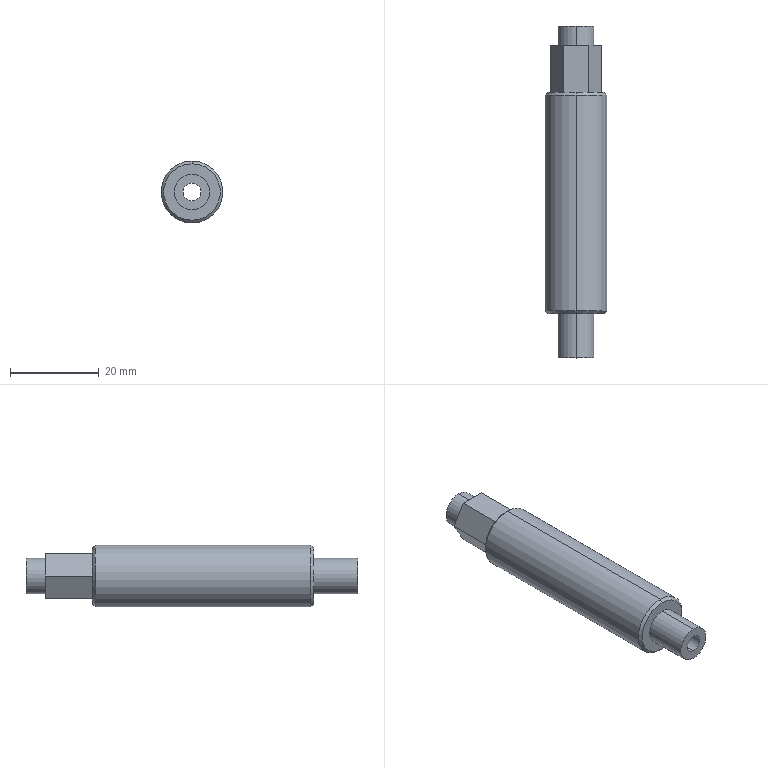Part | SolidWorks | features RefAxis 9, 3DProfileFeature 3, Revolution 2, ICE 1, RevCut 1 | 1 solid | 29 faces | box 14 x 75 x 14 mm | volume 8378 mm3 | plane 11 | cylinder 10 | cone 8 | commonest cylinder face diameters 8 x4 4 x2 4.134 x2 14 x2
STEP:
#1=CARTESIAN_POINT('',(0.,50.,-2.));
#2=VERTEX_POINT('',#1);
#3=CARTESIAN_POINT('',(0.,50.,2.));
#4=VERTEX_POINT('',#3);
#5=CARTESIAN_POINT('',(0.,50.,0.));
#6=DIRECTION('',(0.,1.,0.));
#7=DIRECTION('',(0.,0.,1.));
#8=AXIS2_PLACEMENT_3D('',#5,#6,#7);
#9=CIRCLE('',#8,2.);
#10=EDGE_CURVE('',#2,#4,#9,.T.);
#11=ORIENTED_EDGE('',*,*,#10,.F.);
#12=CARTESIAN_POINT('',(0.,119.961,-2.));
#13=VERTEX_POINT('',#12);
#14=CARTESIAN_POINT('',(0.,50.,-2.));
#15=DIRECTION('',(0.,1.,0.));
#16=VECTOR('',#15,1000.);
#17=LINE('',#14,#16);
#18=EDGE_CURVE('',#2,#13,#17,.T.);
#19=ORIENTED_EDGE('',*,*,#18,.T.);
#20=CARTESIAN_POINT('',(0.,119.961,2.));
#21=VERTEX_POINT('',#20);
#22=CARTESIAN_POINT('',(0.,119.961,0.));
#23=DIRECTION('',(0.,1.,0.));
#24=DIRECTION('',(0.,0.,1.));
#25=AXIS2_PLACEMENT_3D('',#22,#23,#24);
#26=CIRCLE('',#25,2.);
#27=EDGE_CURVE('',#13,#21,#26,.T.);
#28=ORIENTED_EDGE('',*,*,#27,.T.);
#29=CARTESIAN_POINT('',(0.,50.,2.));
#30=DIRECTION('',(0.,1.,0.));
#31=VECTOR('',#30,1000.);
#32=LINE('',#29,#31);
#33=EDGE_CURVE('',#4,#21,#32,.T.);
#34=ORIENTED_EDGE('',*,*,#33,.F.);
#35=EDGE_LOOP('',(#11,#19,#28,#34));
#36=FACE_OUTER_BOUND('',#35,.T.);
#37=CARTESIAN_POINT('',(0.,50.,0.));
#38=DIRECTION('',(0.,1.,0.));
#39=DIRECTION('',(0.,0.,1.));
#40=AXIS2_PLACEMENT_3D('',#37,#38,#39);
#41=CYLINDRICAL_SURFACE('',#40,2.);
#42=ADVANCED_FACE('',(#36),#41,.F.);
#43=ORIENTED_EDGE('',*,*,#27,.F.);
#44=CARTESIAN_POINT('',(0.,120.,-2.067));
#45=VERTEX_POINT('',#44);
#46=CARTESIAN_POINT('',(0.,119.961,-2.));
#47=DIRECTION('',(0.,0.5,-0.866));
#48=VECTOR('',#47,1000.);
#49=LINE('',#46,#48);
#50=EDGE_CURVE('',#13,#45,#49,.T.);
#51=ORIENTED_EDGE('',*,*,#50,.T.);
#52=CARTESIAN_POINT('',(0.,120.,2.067));
#53=VERTEX_POINT('',#52);
#54=CARTESIAN_POINT('',(0.,120.,0.));
#55=DIRECTION('',(0.,1.,0.));
#56=DIRECTION('',(0.,0.,1.));
#57=AXIS2_PLACEMENT_3D('',#54,#55,#56);
#58=CIRCLE('',#57,2.067);
#59=EDGE_CURVE('',#45,#53,#58,.T.);
#60=ORIENTED_EDGE('',*,*,#59,.T.);
#61=CARTESIAN_POINT('',(0.,119.961,2.));
#62=DIRECTION('',(0.,0.5,0.866));
#63=VECTOR('',#62,1000.);
#64=LINE('',#61,#63);
#65=EDGE_CURVE('',#21,#53,#64,.T.);
#66=ORIENTED_EDGE('',*,*,#65,.F.);
#67=EDGE_LOOP('',(#43,#51,#60,#66));
#68=FACE_OUTER_BOUND('',#67,.T.);
#69=CARTESIAN_POINT('',(0.,119.961,0.));
#70=DIRECTION('',(0.,1.,0.));
#71=DIRECTION('',(0.,0.,1.));
#72=AXIS2_PLACEMENT_3D('',#69,#70,#71);
#73=CONICAL_SURFACE('',#72,2.,1.047);
#74=ADVANCED_FACE('',(#68),#73,.F.);
#75=ORIENTED_EDGE('',*,*,#59,.F.);
#76=CARTESIAN_POINT('',(0.,124.567,-2.067));
#77=VERTEX_POINT('',#76);
#78=CARTESIAN_POINT('',(0.,50.,-2.067));
#79=DIRECTION('',(0.,1.,0.));
#80=VECTOR('',#79,1000.);
#81=LINE('',#78,#80);
#82=EDGE_CURVE('',#45,#77,#81,.T.);
#83=ORIENTED_EDGE('',*,*,#82,.T.);
#84=CARTESIAN_POINT('',(0.,124.567,2.067));
#85=VERTEX_POINT('',#84);
#86=CARTESIAN_POINT('',(0.,124.567,0.));
#87=DIRECTION('',(0.,1.,0.));
#88=DIRECTION('',(0.,0.,1.));
#89=AXIS2_PLACEMENT_3D('',#86,#87,#88);
#90=CIRCLE('',#89,2.067);
#91=EDGE_CURVE('',#77,#85,#90,.T.);
#92=ORIENTED_EDGE('',*,*,#91,.T.);
#93=CARTESIAN_POINT('',(0.,50.,2.067));
#94=DIRECTION('',(0.,1.,0.));
#95=VECTOR('',#94,1000.);
#96=LINE('',#93,#95);
#97=EDGE_CURVE('',#53,#85,#96,.T.);
#98=ORIENTED_EDGE('',*,*,#97,.F.);
#99=EDGE_LOOP('',(#75,#83,#92,#98));
#100=FACE_OUTER_BOUND('',#99,.T.);
#101=CARTESIAN_POINT('',(0.,50.,0.));
#102=DIRECTION('',(0.,1.,0.));
#103=DIRECTION('',(0.,0.,1.));
#104=AXIS2_PLACEMENT_3D('',#101,#102,#103);
#105=CYLINDRICAL_SURFACE('',#104,2.067);
#106=ADVANCED_FACE('',(#100),#105,.F.);
#107=ORIENTED_EDGE('',*,*,#91,.F.);
#108=CARTESIAN_POINT('',(0.,125.,-2.5));
#109=VERTEX_POINT('',#108);
#110=CARTESIAN_POINT('',(0.,124.567,-2.067));
#111=DIRECTION('',(0.,0.7071,-0.7071));
#112=VECTOR('',#111,1000.);
#113=LINE('',#110,#112);
#114=EDGE_CURVE('',#77,#109,#113,.T.);
#115=ORIENTED_EDGE('',*,*,#114,.T.);
#116=CARTESIAN_POINT('',(0.,125.,2.5));
#117=VERTEX_POINT('',#116);
#118=CARTESIAN_POINT('',(0.,125.,0.));
#119=DIRECTION('',(0.,1.,0.));
#120=DIRECTION('',(0.,0.,1.));
#121=AXIS2_PLACEMENT_3D('',#118,#119,#120);
#122=CIRCLE('',#121,2.5);
#123=EDGE_CURVE('',#109,#117,#122,.T.);
#124=ORIENTED_EDGE('',*,*,#123,.T.);
#125=CARTESIAN_POINT('',(0.,124.567,2.067));
#126=DIRECTION('',(0.,0.7071,0.7071));
#127=VECTOR('',#126,1000.);
#128=LINE('',#125,#127);
#129=EDGE_CURVE('',#85,#117,#128,.T.);
#130=ORIENTED_EDGE('',*,*,#129,.F.);
#131=EDGE_LOOP('',(#107,#115,#124,#130));
#132=FACE_OUTER_BOUND('',#131,.T.);
#133=CARTESIAN_POINT('',(0.,124.567,0.));
#134=DIRECTION('',(0.,1.,0.));
#135=DIRECTION('',(0.,0.,1.));
#136=AXIS2_PLACEMENT_3D('',#133,#134,#135);
#137=CONICAL_SURFACE('',#136,2.067,0.7854);
#138=ADVANCED_FACE('',(#132),#137,.F.);
#139=CARTESIAN_POINT('',(0.,120.7,4.));
#140=VERTEX_POINT('',#139);
#141=CARTESIAN_POINT('',(0.,120.7,-4.));
#142=VERTEX_POINT('',#141);
#143=CARTESIAN_POINT('',(0.,120.7,0.));
#144=DIRECTION('',(0.,1.,0.));
#145=DIRECTION('',(0.,0.,1.));
#146=AXIS2_PLACEMENT_3D('',#143,#144,#145);
#147=CIRCLE('',#146,4.);
#148=EDGE_CURVE('',#140,#142,#147,.T.);
#149=ORIENTED_EDGE('',*,*,#148,.T.);
#150=CARTESIAN_POINT('',(0.,125.,-4.));
#151=VERTEX_POINT('',#150);
#152=CARTESIAN_POINT('',(0.,120.7,-4.));
#153=DIRECTION('',(0.,1.,0.));
#154=VECTOR('',#153,1000.);
#155=LINE('',#152,#154);
#156=EDGE_CURVE('',#142,#151,#155,.T.);
#157=ORIENTED_EDGE('',*,*,#156,.T.);
#158=CARTESIAN_POINT('',(0.,125.,4.));
#159=VERTEX_POINT('',#158);
#160=CARTESIAN_POINT('',(0.,125.,0.));
#161=DIRECTION('',(0.,1.,0.));
#162=DIRECTION('',(0.,0.,1.));
#163=AXIS2_PLACEMENT_3D('',#160,#161,#162);
#164=CIRCLE('',#163,4.);
#165=EDGE_CURVE('',#159,#151,#164,.T.);
#166=ORIENTED_EDGE('',*,*,#165,.F.);
#167=CARTESIAN_POINT('',(0.,120.7,4.));
#168=DIRECTION('',(0.,1.,0.));
#169=VECTOR('',#168,1000.);
#170=LINE('',#167,#169);
#171=EDGE_CURVE('',#140,#159,#170,.T.);
#172=ORIENTED_EDGE('',*,*,#171,.F.);
#173=EDGE_LOOP('',(#149,#157,#166,#172));
#174=FACE_OUTER_BOUND('',#173,.T.);
#175=CARTESIAN_POINT('',(0.,120.7,0.));
#176=DIRECTION('',(0.,1.,0.));
#177=DIRECTION('',(0.,0.,1.));
#178=AXIS2_PLACEMENT_3D('',#175,#176,#177);
#179=CYLINDRICAL_SURFACE('',#178,4.);
#180=ADVANCED_FACE('',(#174),#179,.T.);
#181=CARTESIAN_POINT('',(0.,50.,4.));
#182=VERTEX_POINT('',#181);
#183=CARTESIAN_POINT('',(0.,50.,-4.));
#184=VERTEX_POINT('',#183);
#185=CARTESIAN_POINT('',(0.,50.,0.));
#186=DIRECTION('',(0.,1.,0.));
#187=DIRECTION('',(0.,0.,1.));
#188=AXIS2_PLACEMENT_3D('',#185,#186,#187);
#189=CIRCLE('',#188,4.);
#190=EDGE_CURVE('',#182,#184,#189,.T.);
#191=ORIENTED_EDGE('',*,*,#190,.T.);
#192=CARTESIAN_POINT('',(0.,60.,-4.));
#193=VERTEX_POINT('',#192);
#194=CARTESIAN_POINT('',(0.,50.,-4.));
#195=DIRECTION('',(0.,1.,0.));
#196=VECTOR('',#195,1000.);
#197=LINE('',#194,#196);
#198=EDGE_CURVE('',#184,#193,#197,.T.);
#199=ORIENTED_EDGE('',*,*,#198,.T.);
#200=CARTESIAN_POINT('',(0.,60.,4.));
#201=VERTEX_POINT('',#200);
#202=CARTESIAN_POINT('',(0.,60.,0.));
#203=DIRECTION('',(0.,1.,0.));
#204=DIRECTION('',(0.,0.,1.));
#205=AXIS2_PLACEMENT_3D('',#202,#203,#204);
#206=CIRCLE('',#205,4.);
#207=EDGE_CURVE('',#201,#193,#206,.T.);
#208=ORIENTED_EDGE('',*,*,#207,.F.);
#209=CARTESIAN_POINT('',(0.,50.,4.));
#210=DIRECTION('',(0.,1.,0.));
#211=VECTOR('',#210,1000.);
#212=LINE('',#209,#211);
#213=EDGE_CURVE('',#182,#201,#212,.T.);
#214=ORIENTED_EDGE('',*,*,#213,.F.);
#215=EDGE_LOOP('',(#191,#199,#208,#214));
#216=FACE_OUTER_BOUND('',#215,.T.);
#217=CARTESIAN_POINT('',(0.,50.,0.));
#218=DIRECTION('',(0.,1.,0.));
#219=DIRECTION('',(0.,0.,1.));
#220=AXIS2_PLACEMENT_3D('',#217,#218,#219);
#221=CYLINDRICAL_SURFACE('',#220,4.);
#222=ADVANCED_FACE('',(#216),#221,.T.);
#223=CARTESIAN_POINT('',(0.,60.,6.386));
#224=VERTEX_POINT('',#223);
#225=CARTESIAN_POINT('',(0.,60.,-6.386));
#226=VERTEX_POINT('',#225);
#227=CARTESIAN_POINT('',(0.,60.,0.));
#228=DIRECTION('',(0.,1.,0.));
#229=DIRECTION('',(0.,0.,1.));
#230=AXIS2_PLACEMENT_3D('',#227,#228,#229);
#231=CIRCLE('',#230,6.386);
#232=EDGE_CURVE('',#224,#226,#231,.T.);
#233=ORIENTED_EDGE('',*,*,#232,.T.);
#234=CARTESIAN_POINT('',(0.,60.614,-7.));
#235=VERTEX_POINT('',#234);
#236=CARTESIAN_POINT('',(0.,60.,-6.386));
#237=DIRECTION('',(0.,0.7071,-0.7071));
#238=VECTOR('',#237,1000.);
#239=LINE('',#236,#238);
#240=EDGE_CURVE('',#226,#235,#239,.T.);
#241=ORIENTED_EDGE('',*,*,#240,.T.);
#242=CARTESIAN_POINT('',(0.,60.614,7.));
#243=VERTEX_POINT('',#242);
#244=CARTESIAN_POINT('',(0.,60.614,0.));
#245=DIRECTION('',(0.,1.,0.));
#246=DIRECTION('',(0.,0.,1.));
#247=AXIS2_PLACEMENT_3D('',#244,#245,#246);
#248=CIRCLE('',#247,7.);
#249=EDGE_CURVE('',#243,#235,#248,.T.);
#250=ORIENTED_EDGE('',*,*,#249,.F.);
#251=CARTESIAN_POINT('',(0.,60.,6.386));
#252=DIRECTION('',(0.,0.7071,0.7071));
#253=VECTOR('',#252,1000.);
#254=LINE('',#251,#253);
#255=EDGE_CURVE('',#224,#243,#254,.T.);
#256=ORIENTED_EDGE('',*,*,#255,.F.);
#257=EDGE_LOOP('',(#233,#241,#250,#256));
#258=FACE_OUTER_BOUND('',#257,.T.);
#259=CARTESIAN_POINT('',(0.,60.,0.));
#260=DIRECTION('',(0.,1.,0.));
#261=DIRECTION('',(0.,0.,1.));
#262=AXIS2_PLACEMENT_3D('',#259,#260,#261);
#263=CONICAL_SURFACE('',#262,6.386,0.7854);
#264=ADVANCED_FACE('',(#258),#263,.T.);
#265=ORIENTED_EDGE('',*,*,#249,.T.);
#266=CARTESIAN_POINT('',(0.,109.386,-7.));
#267=VERTEX_POINT('',#266);
#268=CARTESIAN_POINT('',(0.,50.,-7.));
#269=DIRECTION('',(0.,1.,0.));
#270=VECTOR('',#269,1000.);
#271=LINE('',#268,#270);
#272=EDGE_CURVE('',#235,#267,#271,.T.);
#273=ORIENTED_EDGE('',*,*,#272,.T.);
#274=CARTESIAN_POINT('',(0.,109.386,7.));
#275=VERTEX_POINT('',#274);
#276=CARTESIAN_POINT('',(0.,109.386,0.));
#277=DIRECTION('',(0.,1.,0.));
#278=DIRECTION('',(0.,0.,1.));
#279=AXIS2_PLACEMENT_3D('',#276,#277,#278);
#280=CIRCLE('',#279,7.);
#281=EDGE_CURVE('',#275,#267,#280,.T.);
#282=ORIENTED_EDGE('',*,*,#281,.F.);
#283=CARTESIAN_POINT('',(0.,50.,7.));
#284=DIRECTION('',(0.,1.,0.));
#285=VECTOR('',#284,1000.);
#286=LINE('',#283,#285);
#287=EDGE_CURVE('',#243,#275,#286,.T.);
#288=ORIENTED_EDGE('',*,*,#287,.F.);
#289=EDGE_LOOP('',(#265,#273,#282,#288));
#290=FACE_OUTER_BOUND('',#289,.T.);
#291=CARTESIAN_POINT('',(0.,50.,0.));
#292=DIRECTION('',(0.,1.,0.));
#293=DIRECTION('',(0.,0.,1.));
#294=AXIS2_PLACEMENT_3D('',#291,#292,#293);
#295=CYLINDRICAL_SURFACE('',#294,7.);
#296=ADVANCED_FACE('',(#290),#295,.T.);
#297=CARTESIAN_POINT('',(0.,110.,6.386));
#298=VERTEX_POINT('',#297);
#299=CARTESIAN_POINT('',(0.,110.,-6.386));
#300=VERTEX_POINT('',#299);
#301=CARTESIAN_POINT('',(0.,110.,0.));
#302=DIRECTION('',(0.,1.,0.));
#303=DIRECTION('',(0.,0.,1.));
#304=AXIS2_PLACEMENT_3D('',#301,#302,#303);
#305=CIRCLE('',#304,6.386);
#306=EDGE_CURVE('',#298,#300,#305,.T.);
#307=ORIENTED_EDGE('',*,*,#306,.F.);
#308=CARTESIAN_POINT('',(0.,109.386,7.));
#309=DIRECTION('',(0.,-0.7071,0.7071));
#310=VECTOR('',#309,1000.);
#311=LINE('',#308,#310);
#312=EDGE_CURVE('',#298,#275,#311,.T.);
#313=ORIENTED_EDGE('',*,*,#312,.T.);
#314=ORIENTED_EDGE('',*,*,#281,.T.);
#315=CARTESIAN_POINT('',(0.,109.386,-7.));
#316=DIRECTION('',(0.,-0.7071,-0.7071));
#317=VECTOR('',#316,1000.);
#318=LINE('',#315,#317);
#319=EDGE_CURVE('',#300,#267,#318,.T.);
#320=ORIENTED_EDGE('',*,*,#319,.F.);
#321=EDGE_LOOP('',(#307,#313,#314,#320));
#322=FACE_OUTER_BOUND('',#321,.T.);
#323=CARTESIAN_POINT('',(0.,109.386,0.));
#324=DIRECTION('',(0.,-1.,0.));
#325=DIRECTION('',(0.,0.,-1.));
#326=AXIS2_PLACEMENT_3D('',#323,#324,#325);
#327=CONICAL_SURFACE('',#326,7.,0.7854);
#328=ADVANCED_FACE('',(#322),#327,.T.);
#329=ORIENTED_EDGE('',*,*,#190,.F.);
#330=CARTESIAN_POINT('',(0.,50.,0.));
#331=DIRECTION('',(0.,1.,0.));
#332=DIRECTION('',(0.,0.,1.));
#333=AXIS2_PLACEMENT_3D('',#330,#331,#332);
#334=CIRCLE('',#333,4.);
#335=EDGE_CURVE('',#184,#182,#334,.T.);
#336=ORIENTED_EDGE('',*,*,#335,.F.);
#337=EDGE_LOOP('',(#329,#336));
#338=FACE_OUTER_BOUND('',#337,.T.);
#339=CARTESIAN_POINT('',(0.,50.,0.));
#340=DIRECTION('',(0.,1.,0.));
#341=DIRECTION('',(0.,0.,1.));
#342=AXIS2_PLACEMENT_3D('',#339,#340,#341);
#343=CIRCLE('',#342,2.);
#344=EDGE_CURVE('',#4,#2,#343,.T.);
#345=ORIENTED_EDGE('',*,*,#344,.T.);
#346=ORIENTED_EDGE('',*,*,#10,.T.);
#347=EDGE_LOOP('',(#345,#346));
#348=FACE_BOUND('',#347,.T.);
#349=CARTESIAN_POINT('',(4.,50.,0.));
#350=DIRECTION('',(0.,1.,0.));
#351=DIRECTION('',(0.,0.,1.));
#352=AXIS2_PLACEMENT_3D('',#349,#350,#351);
#353=PLANE('',#352);
#354=ADVANCED_FACE('',(#338,#348),#353,.F.);
#355=ORIENTED_EDGE('',*,*,#165,.T.);
#356=CARTESIAN_POINT('',(0.,125.,0.));
#357=DIRECTION('',(0.,1.,0.));
#358=DIRECTION('',(0.,0.,1.));
#359=AXIS2_PLACEMENT_3D('',#356,#357,#358);
#360=CIRCLE('',#359,4.);
#361=EDGE_CURVE('',#151,#159,#360,.T.);
#362=ORIENTED_EDGE('',*,*,#361,.T.);
#363=EDGE_LOOP('',(#355,#362));
#364=FACE_OUTER_BOUND('',#363,.T.);
#365=CARTESIAN_POINT('',(0.,125.,0.));
#366=DIRECTION('',(0.,1.,0.));
#367=DIRECTION('',(0.,0.,1.));
#368=AXIS2_PLACEMENT_3D('',#365,#366,#367);
#369=CIRCLE('',#368,2.5);
#370=EDGE_CURVE('',#117,#109,#369,.T.);
#371=ORIENTED_EDGE('',*,*,#370,.F.);
#372=ORIENTED_EDGE('',*,*,#123,.F.);
#373=EDGE_LOOP('',(#371,#372));
#374=FACE_BOUND('',#373,.T.);
#375=CARTESIAN_POINT('',(0.,125.,0.));
#376=DIRECTION('',(0.,-1.,0.));
#377=DIRECTION('',(0.,0.,-1.));
#378=AXIS2_PLACEMENT_3D('',#375,#376,#377);
#379=PLANE('',#378);
#380=ADVANCED_FACE('',(#364,#374),#379,.F.);
#381=CARTESIAN_POINT('',(-2.887,120.7,-5.));
#382=VERTEX_POINT('',#381);
#383=CARTESIAN_POINT('',(-5.774,120.7,0.));
#384=VERTEX_POINT('',#383);
#385=CARTESIAN_POINT('',(-2.887,120.7,-5.));
#386=DIRECTION('',(-0.5,0.,0.866));
#387=VECTOR('',#386,1000.);
#388=LINE('',#385,#387);
#389=EDGE_CURVE('',#382,#384,#388,.T.);
#390=ORIENTED_EDGE('',*,*,#389,.T.);
#391=CARTESIAN_POINT('',(-2.887,120.7,5.));
#392=VERTEX_POINT('',#391);
#393=CARTESIAN_POINT('',(-5.774,120.7,0.));
#394=DIRECTION('',(0.5,0.,0.866));
#395=VECTOR('',#394,1000.);
#396=LINE('',#393,#395);
#397=EDGE_CURVE('',#384,#392,#396,.T.);
#398=ORIENTED_EDGE('',*,*,#397,.T.);
#399=CARTESIAN_POINT('',(2.887,120.7,5.));
#400=VERTEX_POINT('',#399);
#401=CARTESIAN_POINT('',(-2.887,120.7,5.));
#402=DIRECTION('',(1.,0.,0.));
#403=VECTOR('',#402,1000.);
#404=LINE('',#401,#403);
#405=EDGE_CURVE('',#392,#400,#404,.T.);
#406=ORIENTED_EDGE('',*,*,#405,.T.);
#407=CARTESIAN_POINT('',(5.774,120.7,0.));
#408=VERTEX_POINT('',#407);
#409=CARTESIAN_POINT('',(2.887,120.7,5.));
#410=DIRECTION('',(0.5,0.,-0.866));
#411=VECTOR('',#410,1000.);
#412=LINE('',#409,#411);
#413=EDGE_CURVE('',#400,#408,#412,.T.);
#414=ORIENTED_EDGE('',*,*,#413,.T.);
#415=CARTESIAN_POINT('',(2.887,120.7,-5.));
#416=VERTEX_POINT('',#415);
#417=CARTESIAN_POINT('',(5.774,120.7,0.));
#418=DIRECTION('',(-0.5,0.,-0.866));
#419=VECTOR('',#418,1000.);
#420=LINE('',#417,#419);
#421=EDGE_CURVE('',#408,#416,#420,.T.);
#422=ORIENTED_EDGE('',*,*,#421,.T.);
#423=CARTESIAN_POINT('',(2.887,120.7,-5.));
#424=DIRECTION('',(-1.,0.,0.));
#425=VECTOR('',#424,1000.);
#426=LINE('',#423,#425);
#427=EDGE_CURVE('',#416,#382,#426,.T.);
#428=ORIENTED_EDGE('',*,*,#427,.T.);
#429=EDGE_LOOP('',(#390,#398,#406,#414,#422,#428));
#430=FACE_OUTER_BOUND('',#429,.T.);
#431=ORIENTED_EDGE('',*,*,#148,.F.);
#432=CARTESIAN_POINT('',(0.,120.7,0.));
#433=DIRECTION('',(0.,1.,0.));
#434=DIRECTION('',(0.,0.,1.));
#435=AXIS2_PLACEMENT_3D('',#432,#433,#434);
#436=CIRCLE('',#435,4.);
#437=EDGE_CURVE('',#142,#140,#436,.T.);
#438=ORIENTED_EDGE('',*,*,#437,.F.);
#439=EDGE_LOOP('',(#431,#438));
#440=FACE_BOUND('',#439,.T.);
#441=CARTESIAN_POINT('',(0.,120.7,0.));
#442=DIRECTION('',(0.,1.,0.));
#443=DIRECTION('',(0.,0.,1.));
#444=AXIS2_PLACEMENT_3D('',#441,#442,#443);
#445=PLANE('',#444);
#446=ADVANCED_FACE('',(#430,#440),#445,.T.);
#447=CARTESIAN_POINT('',(0.,110.,0.));
#448=DIRECTION('',(0.,1.,0.));
#449=DIRECTION('',(0.,0.,1.));
#450=AXIS2_PLACEMENT_3D('',#447,#448,#449);
#451=CIRCLE('',#450,6.386);
#452=EDGE_CURVE('',#300,#298,#451,.T.);
#453=ORIENTED_EDGE('',*,*,#452,.T.);
#454=ORIENTED_EDGE('',*,*,#306,.T.);
#455=EDGE_LOOP('',(#453,#454));
#456=FACE_OUTER_BOUND('',#455,.T.);
#457=CARTESIAN_POINT('',(-2.887,110.,-5.));
#458=VERTEX_POINT('',#457);
#459=CARTESIAN_POINT('',(-5.774,110.,0.));
#460=VERTEX_POINT('',#459);
#461=CARTESIAN_POINT('',(-2.887,110.,-5.));
#462=DIRECTION('',(-0.5,0.,0.866));
#463=VECTOR('',#462,1000.);
#464=LINE('',#461,#463);
#465=EDGE_CURVE('',#458,#460,#464,.T.);
#466=ORIENTED_EDGE('',*,*,#465,.F.);
#467=CARTESIAN_POINT('',(2.887,110.,-5.));
#468=VERTEX_POINT('',#467);
#469=CARTESIAN_POINT('',(2.887,110.,-5.));
#470=DIRECTION('',(-1.,0.,0.));
#471=VECTOR('',#470,1000.);
#472=LINE('',#469,#471);
#473=EDGE_CURVE('',#468,#458,#472,.T.);
#474=ORIENTED_EDGE('',*,*,#473,.F.);
#475=CARTESIAN_POINT('',(5.774,110.,0.));
#476=VERTEX_POINT('',#475);
#477=CARTESIAN_POINT('',(5.774,110.,0.));
#478=DIRECTION('',(-0.5,0.,-0.866));
#479=VECTOR('',#478,1000.);
#480=LINE('',#477,#479);
#481=EDGE_CURVE('',#476,#468,#480,.T.);
#482=ORIENTED_EDGE('',*,*,#481,.F.);
#483=CARTESIAN_POINT('',(2.887,110.,5.));
#484=VERTEX_POINT('',#483);
#485=CARTESIAN_POINT('',(2.887,110.,5.));
#486=DIRECTION('',(0.5,0.,-0.866));
#487=VECTOR('',#486,1000.);
#488=LINE('',#485,#487);
#489=EDGE_CURVE('',#484,#476,#488,.T.);
#490=ORIENTED_EDGE('',*,*,#489,.F.);
#491=CARTESIAN_POINT('',(-2.887,110.,5.));
#492=VERTEX_POINT('',#491);
#493=CARTESIAN_POINT('',(-2.887,110.,5.));
#494=DIRECTION('',(1.,0.,0.));
#495=VECTOR('',#494,1000.);
#496=LINE('',#493,#495);
#497=EDGE_CURVE('',#492,#484,#496,.T.);
#498=ORIENTED_EDGE('',*,*,#497,.F.);
#499=CARTESIAN_POINT('',(-5.774,110.,0.));
#500=DIRECTION('',(0.5,0.,0.866));
#501=VECTOR('',#500,1000.);
#502=LINE('',#499,#501);
#503=EDGE_CURVE('',#460,#492,#502,.T.);
#504=ORIENTED_EDGE('',*,*,#503,.F.);
#505=EDGE_LOOP('',(#466,#474,#482,#490,#498,#504));
#506=FACE_BOUND('',#505,.T.);
#507=CARTESIAN_POINT('',(0.,110.,0.));
#508=DIRECTION('',(0.,-1.,0.));
#509=DIRECTION('',(0.,0.,-1.));
#510=AXIS2_PLACEMENT_3D('',#507,#508,#509);
#511=PLANE('',#510);
#512=ADVANCED_FACE('',(#456,#506),#511,.F.);
#513=ORIENTED_EDGE('',*,*,#312,.F.);
#514=ORIENTED_EDGE('',*,*,#452,.F.);
#515=ORIENTED_EDGE('',*,*,#319,.T.);
#516=CARTESIAN_POINT('',(0.,109.386,0.));
#517=DIRECTION('',(0.,1.,0.));
#518=DIRECTION('',(0.,0.,1.));
#519=AXIS2_PLACEMENT_3D('',#516,#517,#518);
#520=CIRCLE('',#519,7.);
#521=EDGE_CURVE('',#267,#275,#520,.T.);
#522=ORIENTED_EDGE('',*,*,#521,.T.);
#523=EDGE_LOOP('',(#513,#514,#515,#522));
#524=FACE_OUTER_BOUND('',#523,.T.);
#525=CARTESIAN_POINT('',(0.,109.386,0.));
#526=DIRECTION('',(0.,-1.,0.));
#527=DIRECTION('',(0.,0.,-1.));
#528=AXIS2_PLACEMENT_3D('',#525,#526,#527);
#529=CONICAL_SURFACE('',#528,7.,0.7854);
#530=ADVANCED_FACE('',(#524),#529,.T.);
#531=ORIENTED_EDGE('',*,*,#272,.F.);
#532=CARTESIAN_POINT('',(0.,60.614,0.));
#533=DIRECTION('',(0.,1.,0.));
#534=DIRECTION('',(0.,0.,1.));
#535=AXIS2_PLACEMENT_3D('',#532,#533,#534);
#536=CIRCLE('',#535,7.);
#537=EDGE_CURVE('',#235,#243,#536,.T.);
#538=ORIENTED_EDGE('',*,*,#537,.T.);
#539=ORIENTED_EDGE('',*,*,#287,.T.);
#540=ORIENTED_EDGE('',*,*,#521,.F.);
#541=EDGE_LOOP('',(#531,#538,#539,#540));
#542=FACE_OUTER_BOUND('',#541,.T.);
#543=CARTESIAN_POINT('',(0.,50.,0.));
#544=DIRECTION('',(0.,1.,0.));
#545=DIRECTION('',(0.,0.,1.));
#546=AXIS2_PLACEMENT_3D('',#543,#544,#545);
#547=CYLINDRICAL_SURFACE('',#546,7.);
#548=ADVANCED_FACE('',(#542),#547,.T.);
#549=ORIENTED_EDGE('',*,*,#240,.F.);
#550=CARTESIAN_POINT('',(0.,60.,0.));
#551=DIRECTION('',(0.,1.,0.));
#552=DIRECTION('',(0.,0.,1.));
#553=AXIS2_PLACEMENT_3D('',#550,#551,#552);
#554=CIRCLE('',#553,6.386);
#555=EDGE_CURVE('',#226,#224,#554,.T.);
#556=ORIENTED_EDGE('',*,*,#555,.T.);
#557=ORIENTED_EDGE('',*,*,#255,.T.);
#558=ORIENTED_EDGE('',*,*,#537,.F.);
#559=EDGE_LOOP('',(#549,#556,#557,#558));
#560=FACE_OUTER_BOUND('',#559,.T.);
#561=CARTESIAN_POINT('',(0.,60.,0.));
#562=DIRECTION('',(0.,1.,0.));
#563=DIRECTION('',(0.,0.,1.));
#564=AXIS2_PLACEMENT_3D('',#561,#562,#563);
#565=CONICAL_SURFACE('',#564,6.386,0.7854);
#566=ADVANCED_FACE('',(#560),#565,.T.);
#567=ORIENTED_EDGE('',*,*,#232,.F.);
#568=ORIENTED_EDGE('',*,*,#555,.F.);
#569=EDGE_LOOP('',(#567,#568));
#570=FACE_OUTER_BOUND('',#569,.T.);
#571=ORIENTED_EDGE('',*,*,#207,.T.);
#572=CARTESIAN_POINT('',(0.,60.,0.));
#573=DIRECTION('',(0.,1.,0.));
#574=DIRECTION('',(0.,0.,1.));
#575=AXIS2_PLACEMENT_3D('',#572,#573,#574);
#576=CIRCLE('',#575,4.);
#577=EDGE_CURVE('',#193,#201,#576,.T.);
#578=ORIENTED_EDGE('',*,*,#577,.T.);
#579=EDGE_LOOP('',(#571,#578));
#580=FACE_BOUND('',#579,.T.);
#581=CARTESIAN_POINT('',(6.386,60.,0.));
#582=DIRECTION('',(0.,1.,0.));
#583=DIRECTION('',(0.,0.,1.));
#584=AXIS2_PLACEMENT_3D('',#581,#582,#583);
#585=PLANE('',#584);
#586=ADVANCED_FACE('',(#570,#580),#585,.F.);
#587=ORIENTED_EDGE('',*,*,#198,.F.);
#588=ORIENTED_EDGE('',*,*,#335,.T.);
#589=ORIENTED_EDGE('',*,*,#213,.T.);
#590=ORIENTED_EDGE('',*,*,#577,.F.);
#591=EDGE_LOOP('',(#587,#588,#589,#590));
#592=FACE_OUTER_BOUND('',#591,.T.);
#593=CARTESIAN_POINT('',(0.,50.,0.));
#594=DIRECTION('',(0.,1.,0.));
#595=DIRECTION('',(0.,0.,1.));
#596=AXIS2_PLACEMENT_3D('',#593,#594,#595);
#597=CYLINDRICAL_SURFACE('',#596,4.);
#598=ADVANCED_FACE('',(#592),#597,.T.);
#599=ORIENTED_EDGE('',*,*,#465,.T.);
#600=CARTESIAN_POINT('',(-5.774,120.7,0.));
#601=DIRECTION('',(0.,-1.,0.));
#602=VECTOR('',#601,1000.);
#603=LINE('',#600,#602);
#604=EDGE_CURVE('',#384,#460,#603,.T.);
#605=ORIENTED_EDGE('',*,*,#604,.F.);
#606=ORIENTED_EDGE('',*,*,#389,.F.);
#607=CARTESIAN_POINT('',(-2.887,120.7,-5.));
#608=DIRECTION('',(0.,-1.,0.));
#609=VECTOR('',#608,1000.);
#610=LINE('',#607,#609);
#611=EDGE_CURVE('',#382,#458,#610,.T.);
#612=ORIENTED_EDGE('',*,*,#611,.T.);
#613=EDGE_LOOP('',(#599,#605,#606,#612));
#614=FACE_OUTER_BOUND('',#613,.T.);
#615=CARTESIAN_POINT('',(-2.887,120.7,-5.));
#616=DIRECTION('',(0.866,0.,0.5));
#617=DIRECTION('',(0.5,0.,-0.866));
#618=AXIS2_PLACEMENT_3D('',#615,#616,#617);
#619=PLANE('',#618);
#620=ADVANCED_FACE('',(#614),#619,.F.);
#621=ORIENTED_EDGE('',*,*,#503,.T.);
#622=CARTESIAN_POINT('',(-2.887,120.7,5.));
#623=DIRECTION('',(0.,-1.,0.));
#624=VECTOR('',#623,1000.);
#625=LINE('',#622,#624);
#626=EDGE_CURVE('',#392,#492,#625,.T.);
#627=ORIENTED_EDGE('',*,*,#626,.F.);
#628=ORIENTED_EDGE('',*,*,#397,.F.);
#629=ORIENTED_EDGE('',*,*,#604,.T.);
#630=EDGE_LOOP('',(#621,#627,#628,#629));
#631=FACE_OUTER_BOUND('',#630,.T.);
#632=CARTESIAN_POINT('',(-5.774,120.7,0.));
#633=DIRECTION('',(0.866,0.,-0.5));
#634=DIRECTION('',(-0.5,0.,-0.866));
#635=AXIS2_PLACEMENT_3D('',#632,#633,#634);
#636=PLANE('',#635);
#637=ADVANCED_FACE('',(#631),#636,.F.);
#638=ORIENTED_EDGE('',*,*,#497,.T.);
#639=CARTESIAN_POINT('',(2.887,120.7,5.));
#640=DIRECTION('',(0.,-1.,0.));
#641=VECTOR('',#640,1000.);
#642=LINE('',#639,#641);
#643=EDGE_CURVE('',#400,#484,#642,.T.);
#644=ORIENTED_EDGE('',*,*,#643,.F.);
#645=ORIENTED_EDGE('',*,*,#405,.F.);
#646=ORIENTED_EDGE('',*,*,#626,.T.);
#647=EDGE_LOOP('',(#638,#644,#645,#646));
#648=FACE_OUTER_BOUND('',#647,.T.);
#649=CARTESIAN_POINT('',(-2.887,120.7,5.));
#650=DIRECTION('',(0.,0.,-1.));
#651=DIRECTION('',(-1.,0.,0.));
#652=AXIS2_PLACEMENT_3D('',#649,#650,#651);
#653=PLANE('',#652);
#654=ADVANCED_FACE('',(#648),#653,.F.);
#655=ORIENTED_EDGE('',*,*,#489,.T.);
#656=CARTESIAN_POINT('',(5.774,120.7,0.));
#657=DIRECTION('',(0.,-1.,0.));
#658=VECTOR('',#657,1000.);
#659=LINE('',#656,#658);
#660=EDGE_CURVE('',#408,#476,#659,.T.);
#661=ORIENTED_EDGE('',*,*,#660,.F.);
#662=ORIENTED_EDGE('',*,*,#413,.F.);
#663=ORIENTED_EDGE('',*,*,#643,.T.);
#664=EDGE_LOOP('',(#655,#661,#662,#663));
#665=FACE_OUTER_BOUND('',#664,.T.);
#666=CARTESIAN_POINT('',(2.887,120.7,5.));
#667=DIRECTION('',(-0.866,0.,-0.5));
#668=DIRECTION('',(-0.5,0.,0.866));
#669=AXIS2_PLACEMENT_3D('',#666,#667,#668);
#670=PLANE('',#669);
#671=ADVANCED_FACE('',(#665),#670,.F.);
#672=ORIENTED_EDGE('',*,*,#481,.T.);
#673=CARTESIAN_POINT('',(2.887,120.7,-5.));
#674=DIRECTION('',(0.,-1.,0.));
#675=VECTOR('',#674,1000.);
#676=LINE('',#673,#675);
#677=EDGE_CURVE('',#416,#468,#676,.T.);
#678=ORIENTED_EDGE('',*,*,#677,.F.);
#679=ORIENTED_EDGE('',*,*,#421,.F.);
#680=ORIENTED_EDGE('',*,*,#660,.T.);
#681=EDGE_LOOP('',(#672,#678,#679,#680));
#682=FACE_OUTER_BOUND('',#681,.T.);
#683=CARTESIAN_POINT('',(5.774,120.7,0.));
#684=DIRECTION('',(-0.866,0.,0.5));
#685=DIRECTION('',(0.5,0.,0.866));
#686=AXIS2_PLACEMENT_3D('',#683,#684,#685);
#687=PLANE('',#686);
#688=ADVANCED_FACE('',(#682),#687,.F.);
#689=ORIENTED_EDGE('',*,*,#473,.T.);
#690=ORIENTED_EDGE('',*,*,#611,.F.);
#691=ORIENTED_EDGE('',*,*,#427,.F.);
#692=ORIENTED_EDGE('',*,*,#677,.T.);
#693=EDGE_LOOP('',(#689,#690,#691,#692));
#694=FACE_OUTER_BOUND('',#693,.T.);
#695=CARTESIAN_POINT('',(2.887,120.7,-5.));
#696=DIRECTION('',(0.,0.,1.));
#697=DIRECTION('',(1.,0.,0.));
#698=AXIS2_PLACEMENT_3D('',#695,#696,#697);
#699=PLANE('',#698);
#700=ADVANCED_FACE('',(#694),#699,.F.);
#701=ORIENTED_EDGE('',*,*,#156,.F.);
#702=ORIENTED_EDGE('',*,*,#437,.T.);
#703=ORIENTED_EDGE('',*,*,#171,.T.);
#704=ORIENTED_EDGE('',*,*,#361,.F.);
#705=EDGE_LOOP('',(#701,#702,#703,#704));
#706=FACE_OUTER_BOUND('',#705,.T.);
#707=CARTESIAN_POINT('',(0.,120.7,0.));
#708=DIRECTION('',(0.,1.,0.));
#709=DIRECTION('',(0.,0.,1.));
#710=AXIS2_PLACEMENT_3D('',#707,#708,#709);
#711=CYLINDRICAL_SURFACE('',#710,4.);
#712=ADVANCED_FACE('',(#706),#711,.T.);
#713=ORIENTED_EDGE('',*,*,#114,.F.);
#714=CARTESIAN_POINT('',(0.,124.567,0.));
#715=DIRECTION('',(0.,1.,0.));
#716=DIRECTION('',(0.,0.,1.));
#717=AXIS2_PLACEMENT_3D('',#714,#715,#716);
#718=CIRCLE('',#717,2.067);
#719=EDGE_CURVE('',#85,#77,#718,.T.);
#720=ORIENTED_EDGE('',*,*,#719,.F.);
#721=ORIENTED_EDGE('',*,*,#129,.T.);
#722=ORIENTED_EDGE('',*,*,#370,.T.);
#723=EDGE_LOOP('',(#713,#720,#721,#722));
#724=FACE_OUTER_BOUND('',#723,.T.);
#725=CARTESIAN_POINT('',(0.,124.567,0.));
#726=DIRECTION('',(0.,1.,0.));
#727=DIRECTION('',(0.,0.,1.));
#728=AXIS2_PLACEMENT_3D('',#725,#726,#727);
#729=CONICAL_SURFACE('',#728,2.067,0.7854);
#730=ADVANCED_FACE('',(#724),#729,.F.);
#731=ORIENTED_EDGE('',*,*,#82,.F.);
#732=CARTESIAN_POINT('',(0.,120.,0.));
#733=DIRECTION('',(0.,1.,0.));
#734=DIRECTION('',(0.,0.,1.));
#735=AXIS2_PLACEMENT_3D('',#732,#733,#734);
#736=CIRCLE('',#735,2.067);
#737=EDGE_CURVE('',#53,#45,#736,.T.);
#738=ORIENTED_EDGE('',*,*,#737,.F.);
#739=ORIENTED_EDGE('',*,*,#97,.T.);
#740=ORIENTED_EDGE('',*,*,#719,.T.);
#741=EDGE_LOOP('',(#731,#738,#739,#740));
#742=FACE_OUTER_BOUND('',#741,.T.);
#743=CARTESIAN_POINT('',(0.,50.,0.));
#744=DIRECTION('',(0.,1.,0.));
#745=DIRECTION('',(0.,0.,1.));
#746=AXIS2_PLACEMENT_3D('',#743,#744,#745);
#747=CYLINDRICAL_SURFACE('',#746,2.067);
#748=ADVANCED_FACE('',(#742),#747,.F.);
#749=ORIENTED_EDGE('',*,*,#50,.F.);
#750=CARTESIAN_POINT('',(0.,119.961,0.));
#751=DIRECTION('',(0.,1.,0.));
#752=DIRECTION('',(0.,0.,1.));
#753=AXIS2_PLACEMENT_3D('',#750,#751,#752);
#754=CIRCLE('',#753,2.);
#755=EDGE_CURVE('',#21,#13,#754,.T.);
#756=ORIENTED_EDGE('',*,*,#755,.F.);
#757=ORIENTED_EDGE('',*,*,#65,.T.);
#758=ORIENTED_EDGE('',*,*,#737,.T.);
#759=EDGE_LOOP('',(#749,#756,#757,#758));
#760=FACE_OUTER_BOUND('',#759,.T.);
#761=CARTESIAN_POINT('',(0.,119.961,0.));
#762=DIRECTION('',(0.,1.,0.));
#763=DIRECTION('',(0.,0.,1.));
#764=AXIS2_PLACEMENT_3D('',#761,#762,#763);
#765=CONICAL_SURFACE('',#764,2.,1.047);
#766=ADVANCED_FACE('',(#760),#765,.F.);
#767=ORIENTED_EDGE('',*,*,#18,.F.);
#768=ORIENTED_EDGE('',*,*,#344,.F.);
#769=ORIENTED_EDGE('',*,*,#33,.T.);
#770=ORIENTED_EDGE('',*,*,#755,.T.);
#771=EDGE_LOOP('',(#767,#768,#769,#770));
#772=FACE_OUTER_BOUND('',#771,.T.);
#773=CARTESIAN_POINT('',(0.,50.,0.));
#774=DIRECTION('',(0.,1.,0.));
#775=DIRECTION('',(0.,0.,1.));
#776=AXIS2_PLACEMENT_3D('',#773,#774,#775);
#777=CYLINDRICAL_SURFACE('',#776,2.);
#778=ADVANCED_FACE('',(#772),#777,.F.);
#779=CLOSED_SHELL('',(#42,#74,#106,#138,#180,#222,#264,#296,#328,#354,#380,#446,#512,#530,#548,#566,#586,#598,#620,#637,#654,#671,#688,#700,#712,#730,#748,#766,#778));
#780=MANIFOLD_SOLID_BREP('',#779);
#781=CARTESIAN_POINT('',(0.,0.,0.));
#782=DIRECTION('',(0.,0.,1.));
#783=DIRECTION('',(1.,0.,0.));
#784=AXIS2_PLACEMENT_3D('',#781,#782,#783);
#785=(LENGTH_UNIT()NAMED_UNIT(*)SI_UNIT(.MILLI.,.METRE.));
#786=UNCERTAINTY_MEASURE_WITH_UNIT(LENGTH_MEASURE(0.00001),#785,'','');
#787=(NAMED_UNIT(*)PLANE_ANGLE_UNIT()SI_UNIT($,.RADIAN.));
#788=(NAMED_UNIT(*)SI_UNIT($,.STERADIAN.)SOLID_ANGLE_UNIT());
#789=(GEOMETRIC_REPRESENTATION_CONTEXT(3)GLOBAL_UNCERTAINTY_ASSIGNED_CONTEXT((#786))GLOBAL_UNIT_ASSIGNED_CONTEXT((#785,#787,#788))REPRESENTATION_CONTEXT('',''));
#790=ADVANCED_BREP_SHAPE_REPRESENTATION('',(#780,#784),#789);